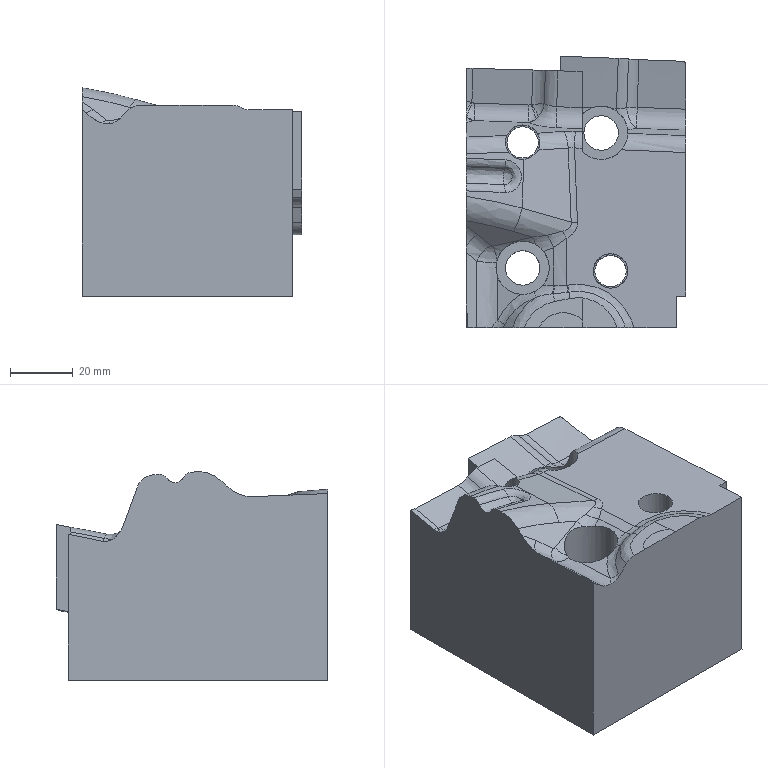Part | NX | features solid 2 | 1 solid | 104 faces | box 70.008 x 86.383 x 66.38 mm | volume 286011 mm3 | spline 83 | plane 13 | cylinder 8 | commonest cylinder face diameters 11 x4 10 x2 17 x2